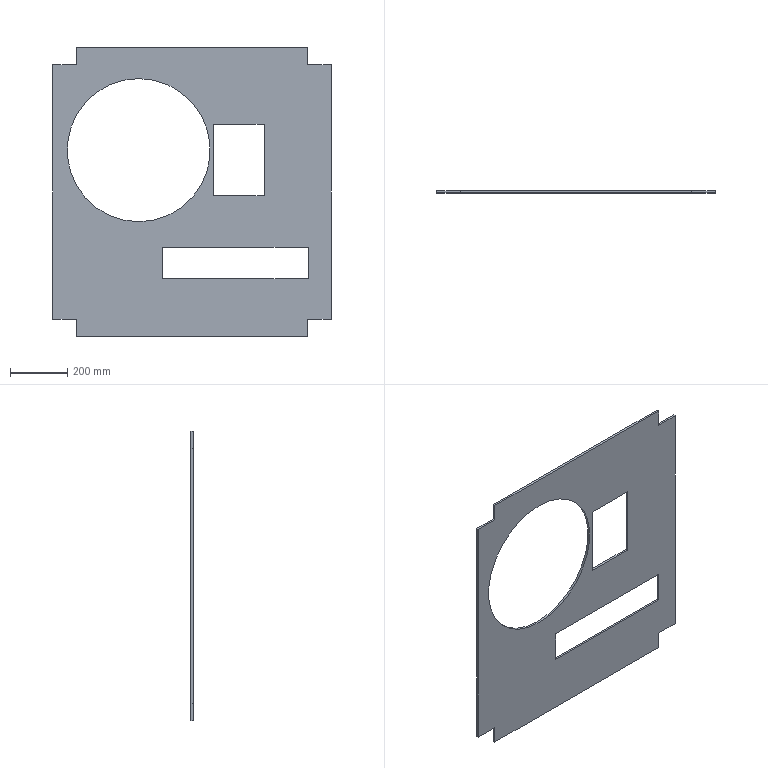Part | STEP file | Guide wheel mechanism revised.sldasm-Part-31 | 1 solid | 24 faces | box 972.42 x 8 x 1012 mm | volume 5346860 mm3 | plane 22 | cylinder 2 | commonest cylinder face diameters 500 x2
STEP:
#1=CARTESIAN_POINT('',(-186.21,820.01,-103.79));
#2=VERTEX_POINT('',#1);
#3=CARTESIAN_POINT('',(-186.21,820.01,396.21));
#4=VERTEX_POINT('',#3);
#5=CARTESIAN_POINT('',(-186.21,820.01,146.21));
#6=DIRECTION('',(0.,1.,0.));
#7=DIRECTION('',(0.,0.,1.));
#8=AXIS2_PLACEMENT_3D('',#5,#6,#7);
#9=CIRCLE('',#8,250.);
#10=EDGE_CURVE('',#2,#4,#9,.T.);
#11=ORIENTED_EDGE('',*,*,#10,.F.);
#12=CARTESIAN_POINT('',(-186.21,828.01,-103.79));
#13=VERTEX_POINT('',#12);
#14=CARTESIAN_POINT('',(-186.21,818.01,-103.79));
#15=DIRECTION('',(0.,1.,0.));
#16=VECTOR('',#15,1000.);
#17=LINE('',#14,#16);
#18=EDGE_CURVE('',#2,#13,#17,.T.);
#19=ORIENTED_EDGE('',*,*,#18,.T.);
#20=CARTESIAN_POINT('',(-186.21,828.01,396.21));
#21=VERTEX_POINT('',#20);
#22=CARTESIAN_POINT('',(-186.21,828.01,146.21));
#23=DIRECTION('',(0.,1.,0.));
#24=DIRECTION('',(0.,0.,1.));
#25=AXIS2_PLACEMENT_3D('',#22,#23,#24);
#26=CIRCLE('',#25,250.);
#27=EDGE_CURVE('',#13,#21,#26,.T.);
#28=ORIENTED_EDGE('',*,*,#27,.T.);
#29=CARTESIAN_POINT('',(-186.21,818.01,396.21));
#30=DIRECTION('',(0.,1.,0.));
#31=VECTOR('',#30,1000.);
#32=LINE('',#29,#31);
#33=EDGE_CURVE('',#4,#21,#32,.T.);
#34=ORIENTED_EDGE('',*,*,#33,.F.);
#35=EDGE_LOOP('',(#11,#19,#28,#34));
#36=FACE_OUTER_BOUND('',#35,.T.);
#37=CARTESIAN_POINT('',(-186.21,818.01,146.21));
#38=DIRECTION('',(0.,1.,0.));
#39=DIRECTION('',(0.,0.,1.));
#40=AXIS2_PLACEMENT_3D('',#37,#38,#39);
#41=CYLINDRICAL_SURFACE('',#40,250.);
#42=ADVANCED_FACE('',(#36),#41,.F.);
#43=CARTESIAN_POINT('',(-404.9,820.01,-506.21));
#44=VERTEX_POINT('',#43);
#45=CARTESIAN_POINT('',(-404.9,820.01,-444.9));
#46=VERTEX_POINT('',#45);
#47=CARTESIAN_POINT('',(-404.9,820.01,-506.21));
#48=DIRECTION('',(0.,0.,1.));
#49=VECTOR('',#48,1000.);
#50=LINE('',#47,#49);
#51=EDGE_CURVE('',#44,#46,#50,.T.);
#52=ORIENTED_EDGE('',*,*,#51,.T.);
#53=CARTESIAN_POINT('',(-404.9,828.01,-444.9));
#54=VERTEX_POINT('',#53);
#55=CARTESIAN_POINT('',(-404.9,828.01,-444.9));
#56=DIRECTION('',(0.,-1.,0.));
#57=VECTOR('',#56,1000.);
#58=LINE('',#55,#57);
#59=EDGE_CURVE('',#54,#46,#58,.T.);
#60=ORIENTED_EDGE('',*,*,#59,.F.);
#61=CARTESIAN_POINT('',(-404.9,828.01,-506.21));
#62=VERTEX_POINT('',#61);
#63=CARTESIAN_POINT('',(-404.9,828.01,-506.21));
#64=DIRECTION('',(0.,0.,1.));
#65=VECTOR('',#64,1000.);
#66=LINE('',#63,#65);
#67=EDGE_CURVE('',#62,#54,#66,.T.);
#68=ORIENTED_EDGE('',*,*,#67,.F.);
#69=CARTESIAN_POINT('',(-404.9,828.01,-506.21));
#70=DIRECTION('',(0.,-1.,0.));
#71=VECTOR('',#70,1000.);
#72=LINE('',#69,#71);
#73=EDGE_CURVE('',#62,#44,#72,.T.);
#74=ORIENTED_EDGE('',*,*,#73,.T.);
#75=EDGE_LOOP('',(#52,#60,#68,#74));
#76=FACE_OUTER_BOUND('',#75,.T.);
#77=CARTESIAN_POINT('',(-404.9,828.01,-506.21));
#78=DIRECTION('',(1.,0.,0.));
#79=DIRECTION('',(0.,0.,-1.));
#80=AXIS2_PLACEMENT_3D('',#77,#78,#79);
#81=PLANE('',#80);
#82=ADVANCED_FACE('',(#76),#81,.F.);
#83=CARTESIAN_POINT('',(-486.21,820.01,-444.9));
#84=VERTEX_POINT('',#83);
#85=CARTESIAN_POINT('',(-404.9,820.01,-444.9));
#86=DIRECTION('',(-1.,0.,0.));
#87=VECTOR('',#86,1000.);
#88=LINE('',#85,#87);
#89=EDGE_CURVE('',#46,#84,#88,.T.);
#90=ORIENTED_EDGE('',*,*,#89,.T.);
#91=CARTESIAN_POINT('',(-486.21,828.01,-444.9));
#92=VERTEX_POINT('',#91);
#93=CARTESIAN_POINT('',(-486.21,828.01,-444.9));
#94=DIRECTION('',(0.,-1.,0.));
#95=VECTOR('',#94,1000.);
#96=LINE('',#93,#95);
#97=EDGE_CURVE('',#92,#84,#96,.T.);
#98=ORIENTED_EDGE('',*,*,#97,.F.);
#99=CARTESIAN_POINT('',(-404.9,828.01,-444.9));
#100=DIRECTION('',(-1.,0.,0.));
#101=VECTOR('',#100,1000.);
#102=LINE('',#99,#101);
#103=EDGE_CURVE('',#54,#92,#102,.T.);
#104=ORIENTED_EDGE('',*,*,#103,.F.);
#105=ORIENTED_EDGE('',*,*,#59,.T.);
#106=EDGE_LOOP('',(#90,#98,#104,#105));
#107=FACE_OUTER_BOUND('',#106,.T.);
#108=CARTESIAN_POINT('',(-404.9,828.01,-444.9));
#109=DIRECTION('',(0.,0.,1.));
#110=DIRECTION('',(1.,0.,0.));
#111=AXIS2_PLACEMENT_3D('',#108,#109,#110);
#112=PLANE('',#111);
#113=ADVANCED_FACE('',(#107),#112,.F.);
#114=CARTESIAN_POINT('',(-486.21,820.01,444.9));
#115=VERTEX_POINT('',#114);
#116=CARTESIAN_POINT('',(-486.21,820.01,-444.9));
#117=DIRECTION('',(0.,0.,1.));
#118=VECTOR('',#117,1000.);
#119=LINE('',#116,#118);
#120=EDGE_CURVE('',#84,#115,#119,.T.);
#121=ORIENTED_EDGE('',*,*,#120,.T.);
#122=CARTESIAN_POINT('',(-486.21,828.01,444.9));
#123=VERTEX_POINT('',#122);
#124=CARTESIAN_POINT('',(-486.21,828.01,444.9));
#125=DIRECTION('',(0.,-1.,0.));
#126=VECTOR('',#125,1000.);
#127=LINE('',#124,#126);
#128=EDGE_CURVE('',#123,#115,#127,.T.);
#129=ORIENTED_EDGE('',*,*,#128,.F.);
#130=CARTESIAN_POINT('',(-486.21,828.01,-444.9));
#131=DIRECTION('',(0.,0.,1.));
#132=VECTOR('',#131,1000.);
#133=LINE('',#130,#132);
#134=EDGE_CURVE('',#92,#123,#133,.T.);
#135=ORIENTED_EDGE('',*,*,#134,.F.);
#136=ORIENTED_EDGE('',*,*,#97,.T.);
#137=EDGE_LOOP('',(#121,#129,#135,#136));
#138=FACE_OUTER_BOUND('',#137,.T.);
#139=CARTESIAN_POINT('',(-486.21,828.01,-444.9));
#140=DIRECTION('',(1.,0.,0.));
#141=DIRECTION('',(0.,0.,-1.));
#142=AXIS2_PLACEMENT_3D('',#139,#140,#141);
#143=PLANE('',#142);
#144=ADVANCED_FACE('',(#138),#143,.F.);
#145=CARTESIAN_POINT('',(-404.9,820.01,444.9));
#146=VERTEX_POINT('',#145);
#147=CARTESIAN_POINT('',(-486.21,820.01,444.9));
#148=DIRECTION('',(1.,0.,0.));
#149=VECTOR('',#148,1000.);
#150=LINE('',#147,#149);
#151=EDGE_CURVE('',#115,#146,#150,.T.);
#152=ORIENTED_EDGE('',*,*,#151,.T.);
#153=CARTESIAN_POINT('',(-404.9,828.01,444.9));
#154=VERTEX_POINT('',#153);
#155=CARTESIAN_POINT('',(-404.9,828.01,444.9));
#156=DIRECTION('',(0.,-1.,0.));
#157=VECTOR('',#156,1000.);
#158=LINE('',#155,#157);
#159=EDGE_CURVE('',#154,#146,#158,.T.);
#160=ORIENTED_EDGE('',*,*,#159,.F.);
#161=CARTESIAN_POINT('',(-486.21,828.01,444.9));
#162=DIRECTION('',(1.,0.,0.));
#163=VECTOR('',#162,1000.);
#164=LINE('',#161,#163);
#165=EDGE_CURVE('',#123,#154,#164,.T.);
#166=ORIENTED_EDGE('',*,*,#165,.F.);
#167=ORIENTED_EDGE('',*,*,#128,.T.);
#168=EDGE_LOOP('',(#152,#160,#166,#167));
#169=FACE_OUTER_BOUND('',#168,.T.);
#170=CARTESIAN_POINT('',(-486.21,828.01,444.9));
#171=DIRECTION('',(0.,0.,-1.));
#172=DIRECTION('',(-1.,0.,0.));
#173=AXIS2_PLACEMENT_3D('',#170,#171,#172);
#174=PLANE('',#173);
#175=ADVANCED_FACE('',(#169),#174,.F.);
#176=CARTESIAN_POINT('',(-404.9,820.01,506.21));
#177=VERTEX_POINT('',#176);
#178=CARTESIAN_POINT('',(-404.9,820.01,444.9));
#179=DIRECTION('',(0.,0.,1.));
#180=VECTOR('',#179,1000.);
#181=LINE('',#178,#180);
#182=EDGE_CURVE('',#146,#177,#181,.T.);
#183=ORIENTED_EDGE('',*,*,#182,.T.);
#184=CARTESIAN_POINT('',(-404.9,828.01,506.21));
#185=VERTEX_POINT('',#184);
#186=CARTESIAN_POINT('',(-404.9,828.01,506.21));
#187=DIRECTION('',(0.,-1.,0.));
#188=VECTOR('',#187,1000.);
#189=LINE('',#186,#188);
#190=EDGE_CURVE('',#185,#177,#189,.T.);
#191=ORIENTED_EDGE('',*,*,#190,.F.);
#192=CARTESIAN_POINT('',(-404.9,828.01,444.9));
#193=DIRECTION('',(0.,0.,1.));
#194=VECTOR('',#193,1000.);
#195=LINE('',#192,#194);
#196=EDGE_CURVE('',#154,#185,#195,.T.);
#197=ORIENTED_EDGE('',*,*,#196,.F.);
#198=ORIENTED_EDGE('',*,*,#159,.T.);
#199=EDGE_LOOP('',(#183,#191,#197,#198));
#200=FACE_OUTER_BOUND('',#199,.T.);
#201=CARTESIAN_POINT('',(-404.9,828.01,444.9));
#202=DIRECTION('',(1.,0.,0.));
#203=DIRECTION('',(0.,0.,-1.));
#204=AXIS2_PLACEMENT_3D('',#201,#202,#203);
#205=PLANE('',#204);
#206=ADVANCED_FACE('',(#200),#205,.F.);
#207=CARTESIAN_POINT('',(404.9,820.01,506.21));
#208=VERTEX_POINT('',#207);
#209=CARTESIAN_POINT('',(0.,820.01,506.21));
#210=DIRECTION('',(1.,0.,0.));
#211=VECTOR('',#210,1000.);
#212=LINE('',#209,#211);
#213=EDGE_CURVE('',#177,#208,#212,.T.);
#214=ORIENTED_EDGE('',*,*,#213,.T.);
#215=CARTESIAN_POINT('',(404.9,828.01,506.21));
#216=VERTEX_POINT('',#215);
#217=CARTESIAN_POINT('',(404.9,828.01,506.21));
#218=DIRECTION('',(0.,-1.,0.));
#219=VECTOR('',#218,1000.);
#220=LINE('',#217,#219);
#221=EDGE_CURVE('',#216,#208,#220,.T.);
#222=ORIENTED_EDGE('',*,*,#221,.F.);
#223=CARTESIAN_POINT('',(-404.9,828.01,506.21));
#224=DIRECTION('',(1.,0.,0.));
#225=VECTOR('',#224,1000.);
#226=LINE('',#223,#225);
#227=EDGE_CURVE('',#185,#216,#226,.T.);
#228=ORIENTED_EDGE('',*,*,#227,.F.);
#229=ORIENTED_EDGE('',*,*,#190,.T.);
#230=EDGE_LOOP('',(#214,#222,#228,#229));
#231=FACE_OUTER_BOUND('',#230,.T.);
#232=CARTESIAN_POINT('',(0.,828.01,506.21));
#233=DIRECTION('',(0.,0.,-1.));
#234=DIRECTION('',(-1.,0.,0.));
#235=AXIS2_PLACEMENT_3D('',#232,#233,#234);
#236=PLANE('',#235);
#237=ADVANCED_FACE('',(#231),#236,.F.);
#238=CARTESIAN_POINT('',(404.9,820.01,444.9));
#239=VERTEX_POINT('',#238);
#240=CARTESIAN_POINT('',(404.9,820.01,506.21));
#241=DIRECTION('',(0.,0.,-1.));
#242=VECTOR('',#241,1000.);
#243=LINE('',#240,#242);
#244=EDGE_CURVE('',#208,#239,#243,.T.);
#245=ORIENTED_EDGE('',*,*,#244,.T.);
#246=CARTESIAN_POINT('',(404.9,828.01,444.9));
#247=VERTEX_POINT('',#246);
#248=CARTESIAN_POINT('',(404.9,828.01,444.9));
#249=DIRECTION('',(0.,-1.,0.));
#250=VECTOR('',#249,1000.);
#251=LINE('',#248,#250);
#252=EDGE_CURVE('',#247,#239,#251,.T.);
#253=ORIENTED_EDGE('',*,*,#252,.F.);
#254=CARTESIAN_POINT('',(404.9,828.01,506.21));
#255=DIRECTION('',(0.,0.,-1.));
#256=VECTOR('',#255,1000.);
#257=LINE('',#254,#256);
#258=EDGE_CURVE('',#216,#247,#257,.T.);
#259=ORIENTED_EDGE('',*,*,#258,.F.);
#260=ORIENTED_EDGE('',*,*,#221,.T.);
#261=EDGE_LOOP('',(#245,#253,#259,#260));
#262=FACE_OUTER_BOUND('',#261,.T.);
#263=CARTESIAN_POINT('',(404.9,828.01,506.21));
#264=DIRECTION('',(-1.,0.,0.));
#265=DIRECTION('',(0.,0.,1.));
#266=AXIS2_PLACEMENT_3D('',#263,#264,#265);
#267=PLANE('',#266);
#268=ADVANCED_FACE('',(#262),#267,.F.);
#269=CARTESIAN_POINT('',(486.21,820.01,444.9));
#270=VERTEX_POINT('',#269);
#271=CARTESIAN_POINT('',(404.9,820.01,444.9));
#272=DIRECTION('',(1.,0.,0.));
#273=VECTOR('',#272,1000.);
#274=LINE('',#271,#273);
#275=EDGE_CURVE('',#239,#270,#274,.T.);
#276=ORIENTED_EDGE('',*,*,#275,.T.);
#277=CARTESIAN_POINT('',(486.21,828.01,444.9));
#278=VERTEX_POINT('',#277);
#279=CARTESIAN_POINT('',(486.21,828.01,444.9));
#280=DIRECTION('',(0.,-1.,0.));
#281=VECTOR('',#280,1000.);
#282=LINE('',#279,#281);
#283=EDGE_CURVE('',#278,#270,#282,.T.);
#284=ORIENTED_EDGE('',*,*,#283,.F.);
#285=CARTESIAN_POINT('',(404.9,828.01,444.9));
#286=DIRECTION('',(1.,0.,0.));
#287=VECTOR('',#286,1000.);
#288=LINE('',#285,#287);
#289=EDGE_CURVE('',#247,#278,#288,.T.);
#290=ORIENTED_EDGE('',*,*,#289,.F.);
#291=ORIENTED_EDGE('',*,*,#252,.T.);
#292=EDGE_LOOP('',(#276,#284,#290,#291));
#293=FACE_OUTER_BOUND('',#292,.T.);
#294=CARTESIAN_POINT('',(404.9,828.01,444.9));
#295=DIRECTION('',(0.,0.,-1.));
#296=DIRECTION('',(-1.,0.,0.));
#297=AXIS2_PLACEMENT_3D('',#294,#295,#296);
#298=PLANE('',#297);
#299=ADVANCED_FACE('',(#293),#298,.F.);
#300=CARTESIAN_POINT('',(486.21,820.01,-444.9));
#301=VERTEX_POINT('',#300);
#302=CARTESIAN_POINT('',(486.21,820.01,444.9));
#303=DIRECTION('',(0.,0.,-1.));
#304=VECTOR('',#303,1000.);
#305=LINE('',#302,#304);
#306=EDGE_CURVE('',#270,#301,#305,.T.);
#307=ORIENTED_EDGE('',*,*,#306,.T.);
#308=CARTESIAN_POINT('',(486.21,828.01,-444.9));
#309=VERTEX_POINT('',#308);
#310=CARTESIAN_POINT('',(486.21,828.01,-444.9));
#311=DIRECTION('',(0.,-1.,0.));
#312=VECTOR('',#311,1000.);
#313=LINE('',#310,#312);
#314=EDGE_CURVE('',#309,#301,#313,.T.);
#315=ORIENTED_EDGE('',*,*,#314,.F.);
#316=CARTESIAN_POINT('',(486.21,828.01,444.9));
#317=DIRECTION('',(0.,0.,-1.));
#318=VECTOR('',#317,1000.);
#319=LINE('',#316,#318);
#320=EDGE_CURVE('',#278,#309,#319,.T.);
#321=ORIENTED_EDGE('',*,*,#320,.F.);
#322=ORIENTED_EDGE('',*,*,#283,.T.);
#323=EDGE_LOOP('',(#307,#315,#321,#322));
#324=FACE_OUTER_BOUND('',#323,.T.);
#325=CARTESIAN_POINT('',(486.21,828.01,444.9));
#326=DIRECTION('',(-1.,0.,0.));
#327=DIRECTION('',(0.,0.,1.));
#328=AXIS2_PLACEMENT_3D('',#325,#326,#327);
#329=PLANE('',#328);
#330=ADVANCED_FACE('',(#324),#329,.F.);
#331=CARTESIAN_POINT('',(404.9,820.01,-444.9));
#332=VERTEX_POINT('',#331);
#333=CARTESIAN_POINT('',(486.21,820.01,-444.9));
#334=DIRECTION('',(-1.,0.,0.));
#335=VECTOR('',#334,1000.);
#336=LINE('',#333,#335);
#337=EDGE_CURVE('',#301,#332,#336,.T.);
#338=ORIENTED_EDGE('',*,*,#337,.T.);
#339=CARTESIAN_POINT('',(404.9,828.01,-444.9));
#340=VERTEX_POINT('',#339);
#341=CARTESIAN_POINT('',(404.9,828.01,-444.9));
#342=DIRECTION('',(0.,-1.,0.));
#343=VECTOR('',#342,1000.);
#344=LINE('',#341,#343);
#345=EDGE_CURVE('',#340,#332,#344,.T.);
#346=ORIENTED_EDGE('',*,*,#345,.F.);
#347=CARTESIAN_POINT('',(486.21,828.01,-444.9));
#348=DIRECTION('',(-1.,0.,0.));
#349=VECTOR('',#348,1000.);
#350=LINE('',#347,#349);
#351=EDGE_CURVE('',#309,#340,#350,.T.);
#352=ORIENTED_EDGE('',*,*,#351,.F.);
#353=ORIENTED_EDGE('',*,*,#314,.T.);
#354=EDGE_LOOP('',(#338,#346,#352,#353));
#355=FACE_OUTER_BOUND('',#354,.T.);
#356=CARTESIAN_POINT('',(486.21,828.01,-444.9));
#357=DIRECTION('',(0.,0.,1.));
#358=DIRECTION('',(1.,0.,0.));
#359=AXIS2_PLACEMENT_3D('',#356,#357,#358);
#360=PLANE('',#359);
#361=ADVANCED_FACE('',(#355),#360,.F.);
#362=CARTESIAN_POINT('',(404.9,820.01,-506.21));
#363=VERTEX_POINT('',#362);
#364=CARTESIAN_POINT('',(404.9,820.01,-444.9));
#365=DIRECTION('',(0.,0.,-1.));
#366=VECTOR('',#365,1000.);
#367=LINE('',#364,#366);
#368=EDGE_CURVE('',#332,#363,#367,.T.);
#369=ORIENTED_EDGE('',*,*,#368,.T.);
#370=CARTESIAN_POINT('',(404.9,828.01,-506.21));
#371=VERTEX_POINT('',#370);
#372=CARTESIAN_POINT('',(404.9,828.01,-506.21));
#373=DIRECTION('',(0.,-1.,0.));
#374=VECTOR('',#373,1000.);
#375=LINE('',#372,#374);
#376=EDGE_CURVE('',#371,#363,#375,.T.);
#377=ORIENTED_EDGE('',*,*,#376,.F.);
#378=CARTESIAN_POINT('',(404.9,828.01,-444.9));
#379=DIRECTION('',(0.,0.,-1.));
#380=VECTOR('',#379,1000.);
#381=LINE('',#378,#380);
#382=EDGE_CURVE('',#340,#371,#381,.T.);
#383=ORIENTED_EDGE('',*,*,#382,.F.);
#384=ORIENTED_EDGE('',*,*,#345,.T.);
#385=EDGE_LOOP('',(#369,#377,#383,#384));
#386=FACE_OUTER_BOUND('',#385,.T.);
#387=CARTESIAN_POINT('',(404.9,828.01,-444.9));
#388=DIRECTION('',(-1.,0.,0.));
#389=DIRECTION('',(0.,0.,1.));
#390=AXIS2_PLACEMENT_3D('',#387,#388,#389);
#391=PLANE('',#390);
#392=ADVANCED_FACE('',(#386),#391,.F.);
#393=CARTESIAN_POINT('',(0.,820.01,-506.21));
#394=DIRECTION('',(-1.,0.,0.));
#395=VECTOR('',#394,1000.);
#396=LINE('',#393,#395);
#397=EDGE_CURVE('',#363,#44,#396,.T.);
#398=ORIENTED_EDGE('',*,*,#397,.T.);
#399=ORIENTED_EDGE('',*,*,#73,.F.);
#400=CARTESIAN_POINT('',(0.,828.01,-506.21));
#401=DIRECTION('',(-1.,0.,0.));
#402=VECTOR('',#401,1000.);
#403=LINE('',#400,#402);
#404=EDGE_CURVE('',#371,#62,#403,.T.);
#405=ORIENTED_EDGE('',*,*,#404,.F.);
#406=ORIENTED_EDGE('',*,*,#376,.T.);
#407=EDGE_LOOP('',(#398,#399,#405,#406));
#408=FACE_OUTER_BOUND('',#407,.T.);
#409=CARTESIAN_POINT('',(0.,828.01,-506.21));
#410=DIRECTION('',(0.,0.,1.));
#411=DIRECTION('',(1.,0.,0.));
#412=AXIS2_PLACEMENT_3D('',#409,#410,#411);
#413=PLANE('',#412);
#414=ADVANCED_FACE('',(#408),#413,.F.);
#415=CARTESIAN_POINT('',(76.71,828.01,-12.79));
#416=VERTEX_POINT('',#415);
#417=CARTESIAN_POINT('',(76.71,828.01,237.21));
#418=VERTEX_POINT('',#417);
#419=CARTESIAN_POINT('',(76.71,828.01,-12.79));
#420=DIRECTION('',(0.,0.,1.));
#421=VECTOR('',#420,1000.);
#422=LINE('',#419,#421);
#423=EDGE_CURVE('',#416,#418,#422,.T.);
#424=ORIENTED_EDGE('',*,*,#423,.F.);
#425=CARTESIAN_POINT('',(251.71,828.01,-12.79));
#426=VERTEX_POINT('',#425);
#427=CARTESIAN_POINT('',(76.71,828.01,-12.79));
#428=DIRECTION('',(-1.,0.,0.));
#429=VECTOR('',#428,1000.);
#430=LINE('',#427,#429);
#431=EDGE_CURVE('',#426,#416,#430,.T.);
#432=ORIENTED_EDGE('',*,*,#431,.F.);
#433=CARTESIAN_POINT('',(251.71,828.01,237.21));
#434=VERTEX_POINT('',#433);
#435=CARTESIAN_POINT('',(251.71,828.01,-12.79));
#436=DIRECTION('',(0.,0.,-1.));
#437=VECTOR('',#436,1000.);
#438=LINE('',#435,#437);
#439=EDGE_CURVE('',#434,#426,#438,.T.);
#440=ORIENTED_EDGE('',*,*,#439,.F.);
#441=CARTESIAN_POINT('',(76.71,828.01,237.21));
#442=DIRECTION('',(1.,0.,0.));
#443=VECTOR('',#442,1000.);
#444=LINE('',#441,#443);
#445=EDGE_CURVE('',#418,#434,#444,.T.);
#446=ORIENTED_EDGE('',*,*,#445,.F.);
#447=EDGE_LOOP('',(#424,#432,#440,#446));
#448=FACE_BOUND('',#447,.T.);
#449=CARTESIAN_POINT('',(406.21,828.01,-193.79));
#450=VERTEX_POINT('',#449);
#451=CARTESIAN_POINT('',(406.21,828.01,-303.79));
#452=VERTEX_POINT('',#451);
#453=CARTESIAN_POINT('',(406.21,828.01,-303.79));
#454=DIRECTION('',(0.,0.,-1.));
#455=VECTOR('',#454,1000.);
#456=LINE('',#453,#455);
#457=EDGE_CURVE('',#450,#452,#456,.T.);
#458=ORIENTED_EDGE('',*,*,#457,.F.);
#459=CARTESIAN_POINT('',(-103.79,828.01,-193.79));
#460=VERTEX_POINT('',#459);
#461=CARTESIAN_POINT('',(406.21,828.01,-193.79));
#462=DIRECTION('',(1.,0.,0.));
#463=VECTOR('',#462,1000.);
#464=LINE('',#461,#463);
#465=EDGE_CURVE('',#460,#450,#464,.T.);
#466=ORIENTED_EDGE('',*,*,#465,.F.);
#467=CARTESIAN_POINT('',(-103.79,828.01,-303.79));
#468=VERTEX_POINT('',#467);
#469=CARTESIAN_POINT('',(-103.79,828.01,-303.79));
#470=DIRECTION('',(0.,0.,1.));
#471=VECTOR('',#470,1000.);
#472=LINE('',#469,#471);
#473=EDGE_CURVE('',#468,#460,#472,.T.);
#474=ORIENTED_EDGE('',*,*,#473,.F.);
#475=CARTESIAN_POINT('',(406.21,828.01,-303.79));
#476=DIRECTION('',(-1.,0.,0.));
#477=VECTOR('',#476,1000.);
#478=LINE('',#475,#477);
#479=EDGE_CURVE('',#452,#468,#478,.T.);
#480=ORIENTED_EDGE('',*,*,#479,.F.);
#481=EDGE_LOOP('',(#458,#466,#474,#480));
#482=FACE_BOUND('',#481,.T.);
#483=CARTESIAN_POINT('',(-186.21,828.01,146.21));
#484=DIRECTION('',(0.,1.,0.));
#485=DIRECTION('',(0.,0.,1.));
#486=AXIS2_PLACEMENT_3D('',#483,#484,#485);
#487=CIRCLE('',#486,250.);
#488=EDGE_CURVE('',#21,#13,#487,.T.);
#489=ORIENTED_EDGE('',*,*,#488,.F.);
#490=ORIENTED_EDGE('',*,*,#27,.F.);
#491=EDGE_LOOP('',(#489,#490));
#492=FACE_BOUND('',#491,.T.);
#493=ORIENTED_EDGE('',*,*,#404,.T.);
#494=ORIENTED_EDGE('',*,*,#67,.T.);
#495=ORIENTED_EDGE('',*,*,#103,.T.);
#496=ORIENTED_EDGE('',*,*,#134,.T.);
#497=ORIENTED_EDGE('',*,*,#165,.T.);
#498=ORIENTED_EDGE('',*,*,#196,.T.);
#499=ORIENTED_EDGE('',*,*,#227,.T.);
#500=ORIENTED_EDGE('',*,*,#258,.T.);
#501=ORIENTED_EDGE('',*,*,#289,.T.);
#502=ORIENTED_EDGE('',*,*,#320,.T.);
#503=ORIENTED_EDGE('',*,*,#351,.T.);
#504=ORIENTED_EDGE('',*,*,#382,.T.);
#505=EDGE_LOOP('',(#493,#494,#495,#496,#497,#498,#499,#500,#501,#502,#503,#504));
#506=FACE_OUTER_BOUND('',#505,.T.);
#507=CARTESIAN_POINT('',(0.,828.01,0.));
#508=DIRECTION('',(0.,1.,0.));
#509=DIRECTION('',(0.,0.,1.));
#510=AXIS2_PLACEMENT_3D('',#507,#508,#509);
#511=PLANE('',#510);
#512=ADVANCED_FACE('',(#448,#482,#492,#506),#511,.T.);
#513=CARTESIAN_POINT('',(76.71,820.01,-12.79));
#514=VERTEX_POINT('',#513);
#515=CARTESIAN_POINT('',(251.71,820.01,-12.79));
#516=VERTEX_POINT('',#515);
#517=CARTESIAN_POINT('',(76.71,820.01,-12.79));
#518=DIRECTION('',(1.,0.,0.));
#519=VECTOR('',#518,1000.);
#520=LINE('',#517,#519);
#521=EDGE_CURVE('',#514,#516,#520,.T.);
#522=ORIENTED_EDGE('',*,*,#521,.F.);
#523=CARTESIAN_POINT('',(76.71,820.01,237.21));
#524=VERTEX_POINT('',#523);
#525=CARTESIAN_POINT('',(76.71,820.01,-12.79));
#526=DIRECTION('',(0.,0.,-1.));
#527=VECTOR('',#526,1000.);
#528=LINE('',#525,#527);
#529=EDGE_CURVE('',#524,#514,#528,.T.);
#530=ORIENTED_EDGE('',*,*,#529,.F.);
#531=CARTESIAN_POINT('',(251.71,820.01,237.21));
#532=VERTEX_POINT('',#531);
#533=CARTESIAN_POINT('',(76.71,820.01,237.21));
#534=DIRECTION('',(-1.,0.,0.));
#535=VECTOR('',#534,1000.);
#536=LINE('',#533,#535);
#537=EDGE_CURVE('',#532,#524,#536,.T.);
#538=ORIENTED_EDGE('',*,*,#537,.F.);
#539=CARTESIAN_POINT('',(251.71,820.01,-12.79));
#540=DIRECTION('',(0.,0.,1.));
#541=VECTOR('',#540,1000.);
#542=LINE('',#539,#541);
#543=EDGE_CURVE('',#516,#532,#542,.T.);
#544=ORIENTED_EDGE('',*,*,#543,.F.);
#545=EDGE_LOOP('',(#522,#530,#538,#544));
#546=FACE_BOUND('',#545,.T.);
#547=CARTESIAN_POINT('',(406.21,820.01,-193.79));
#548=VERTEX_POINT('',#547);
#549=CARTESIAN_POINT('',(-103.79,820.01,-193.79));
#550=VERTEX_POINT('',#549);
#551=CARTESIAN_POINT('',(406.21,820.01,-193.79));
#552=DIRECTION('',(-1.,0.,0.));
#553=VECTOR('',#552,1000.);
#554=LINE('',#551,#553);
#555=EDGE_CURVE('',#548,#550,#554,.T.);
#556=ORIENTED_EDGE('',*,*,#555,.F.);
#557=CARTESIAN_POINT('',(406.21,820.01,-303.79));
#558=VERTEX_POINT('',#557);
#559=CARTESIAN_POINT('',(406.21,820.01,-303.79));
#560=DIRECTION('',(0.,0.,1.));
#561=VECTOR('',#560,1000.);
#562=LINE('',#559,#561);
#563=EDGE_CURVE('',#558,#548,#562,.T.);
#564=ORIENTED_EDGE('',*,*,#563,.F.);
#565=CARTESIAN_POINT('',(-103.79,820.01,-303.79));
#566=VERTEX_POINT('',#565);
#567=CARTESIAN_POINT('',(406.21,820.01,-303.79));
#568=DIRECTION('',(1.,0.,0.));
#569=VECTOR('',#568,1000.);
#570=LINE('',#567,#569);
#571=EDGE_CURVE('',#566,#558,#570,.T.);
#572=ORIENTED_EDGE('',*,*,#571,.F.);
#573=CARTESIAN_POINT('',(-103.79,820.01,-303.79));
#574=DIRECTION('',(0.,0.,-1.));
#575=VECTOR('',#574,1000.);
#576=LINE('',#573,#575);
#577=EDGE_CURVE('',#550,#566,#576,.T.);
#578=ORIENTED_EDGE('',*,*,#577,.F.);
#579=EDGE_LOOP('',(#556,#564,#572,#578));
#580=FACE_BOUND('',#579,.T.);
#581=CARTESIAN_POINT('',(-186.21,820.01,146.21));
#582=DIRECTION('',(0.,1.,0.));
#583=DIRECTION('',(0.,0.,1.));
#584=AXIS2_PLACEMENT_3D('',#581,#582,#583);
#585=CIRCLE('',#584,250.);
#586=EDGE_CURVE('',#4,#2,#585,.T.);
#587=ORIENTED_EDGE('',*,*,#586,.T.);
#588=ORIENTED_EDGE('',*,*,#10,.T.);
#589=EDGE_LOOP('',(#587,#588));
#590=FACE_BOUND('',#589,.T.);
#591=ORIENTED_EDGE('',*,*,#51,.F.);
#592=ORIENTED_EDGE('',*,*,#397,.F.);
#593=ORIENTED_EDGE('',*,*,#368,.F.);
#594=ORIENTED_EDGE('',*,*,#337,.F.);
#595=ORIENTED_EDGE('',*,*,#306,.F.);
#596=ORIENTED_EDGE('',*,*,#275,.F.);
#597=ORIENTED_EDGE('',*,*,#244,.F.);
#598=ORIENTED_EDGE('',*,*,#213,.F.);
#599=ORIENTED_EDGE('',*,*,#182,.F.);
#600=ORIENTED_EDGE('',*,*,#151,.F.);
#601=ORIENTED_EDGE('',*,*,#120,.F.);
#602=ORIENTED_EDGE('',*,*,#89,.F.);
#603=EDGE_LOOP('',(#591,#592,#593,#594,#595,#596,#597,#598,#599,#600,#601,#602));
#604=FACE_OUTER_BOUND('',#603,.T.);
#605=CARTESIAN_POINT('',(0.,820.01,0.));
#606=DIRECTION('',(0.,1.,0.));
#607=DIRECTION('',(0.,0.,1.));
#608=AXIS2_PLACEMENT_3D('',#605,#606,#607);
#609=PLANE('',#608);
#610=ADVANCED_FACE('',(#546,#580,#590,#604),#609,.F.);
#611=ORIENTED_EDGE('',*,*,#18,.F.);
#612=ORIENTED_EDGE('',*,*,#586,.F.);
#613=ORIENTED_EDGE('',*,*,#33,.T.);
#614=ORIENTED_EDGE('',*,*,#488,.T.);
#615=EDGE_LOOP('',(#611,#612,#613,#614));
#616=FACE_OUTER_BOUND('',#615,.T.);
#617=CARTESIAN_POINT('',(-186.21,818.01,146.21));
#618=DIRECTION('',(0.,1.,0.));
#619=DIRECTION('',(0.,0.,1.));
#620=AXIS2_PLACEMENT_3D('',#617,#618,#619);
#621=CYLINDRICAL_SURFACE('',#620,250.);
#622=ADVANCED_FACE('',(#616),#621,.F.);
#623=ORIENTED_EDGE('',*,*,#563,.T.);
#624=CARTESIAN_POINT('',(406.21,-60.001,-193.79));
#625=DIRECTION('',(0.,1.,0.));
#626=VECTOR('',#625,1000.);
#627=LINE('',#624,#626);
#628=EDGE_CURVE('',#548,#450,#627,.T.);
#629=ORIENTED_EDGE('',*,*,#628,.T.);
#630=ORIENTED_EDGE('',*,*,#457,.T.);
#631=CARTESIAN_POINT('',(406.21,-60.001,-303.79));
#632=DIRECTION('',(0.,1.,0.));
#633=VECTOR('',#632,1000.);
#634=LINE('',#631,#633);
#635=EDGE_CURVE('',#558,#452,#634,.T.);
#636=ORIENTED_EDGE('',*,*,#635,.F.);
#637=EDGE_LOOP('',(#623,#629,#630,#636));
#638=FACE_OUTER_BOUND('',#637,.T.);
#639=CARTESIAN_POINT('',(406.21,-60.001,-303.79));
#640=DIRECTION('',(1.,0.,0.));
#641=DIRECTION('',(0.,0.,-1.));
#642=AXIS2_PLACEMENT_3D('',#639,#640,#641);
#643=PLANE('',#642);
#644=ADVANCED_FACE('',(#638),#643,.F.);
#645=ORIENTED_EDGE('',*,*,#555,.T.);
#646=CARTESIAN_POINT('',(-103.79,-60.001,-193.79));
#647=DIRECTION('',(0.,1.,0.));
#648=VECTOR('',#647,1000.);
#649=LINE('',#646,#648);
#650=EDGE_CURVE('',#550,#460,#649,.T.);
#651=ORIENTED_EDGE('',*,*,#650,.T.);
#652=ORIENTED_EDGE('',*,*,#465,.T.);
#653=ORIENTED_EDGE('',*,*,#628,.F.);
#654=EDGE_LOOP('',(#645,#651,#652,#653));
#655=FACE_OUTER_BOUND('',#654,.T.);
#656=CARTESIAN_POINT('',(406.21,-60.001,-193.79));
#657=DIRECTION('',(0.,0.,1.));
#658=DIRECTION('',(1.,0.,0.));
#659=AXIS2_PLACEMENT_3D('',#656,#657,#658);
#660=PLANE('',#659);
#661=ADVANCED_FACE('',(#655),#660,.F.);
#662=ORIENTED_EDGE('',*,*,#577,.T.);
#663=CARTESIAN_POINT('',(-103.79,-60.001,-303.79));
#664=DIRECTION('',(0.,1.,0.));
#665=VECTOR('',#664,1000.);
#666=LINE('',#663,#665);
#667=EDGE_CURVE('',#566,#468,#666,.T.);
#668=ORIENTED_EDGE('',*,*,#667,.T.);
#669=ORIENTED_EDGE('',*,*,#473,.T.);
#670=ORIENTED_EDGE('',*,*,#650,.F.);
#671=EDGE_LOOP('',(#662,#668,#669,#670));
#672=FACE_OUTER_BOUND('',#671,.T.);
#673=CARTESIAN_POINT('',(-103.79,-60.001,-303.79));
#674=DIRECTION('',(-1.,0.,0.));
#675=DIRECTION('',(0.,0.,1.));
#676=AXIS2_PLACEMENT_3D('',#673,#674,#675);
#677=PLANE('',#676);
#678=ADVANCED_FACE('',(#672),#677,.F.);
#679=ORIENTED_EDGE('',*,*,#571,.T.);
#680=ORIENTED_EDGE('',*,*,#635,.T.);
#681=ORIENTED_EDGE('',*,*,#479,.T.);
#682=ORIENTED_EDGE('',*,*,#667,.F.);
#683=EDGE_LOOP('',(#679,#680,#681,#682));
#684=FACE_OUTER_BOUND('',#683,.T.);
#685=CARTESIAN_POINT('',(406.21,-60.001,-303.79));
#686=DIRECTION('',(0.,0.,-1.));
#687=DIRECTION('',(-1.,0.,0.));
#688=AXIS2_PLACEMENT_3D('',#685,#686,#687);
#689=PLANE('',#688);
#690=ADVANCED_FACE('',(#684),#689,.F.);
#691=ORIENTED_EDGE('',*,*,#529,.T.);
#692=CARTESIAN_POINT('',(76.71,-60.001,-12.79));
#693=DIRECTION('',(0.,1.,0.));
#694=VECTOR('',#693,1000.);
#695=LINE('',#692,#694);
#696=EDGE_CURVE('',#514,#416,#695,.T.);
#697=ORIENTED_EDGE('',*,*,#696,.T.);
#698=ORIENTED_EDGE('',*,*,#423,.T.);
#699=CARTESIAN_POINT('',(76.71,-60.001,237.21));
#700=DIRECTION('',(0.,1.,0.));
#701=VECTOR('',#700,1000.);
#702=LINE('',#699,#701);
#703=EDGE_CURVE('',#524,#418,#702,.T.);
#704=ORIENTED_EDGE('',*,*,#703,.F.);
#705=EDGE_LOOP('',(#691,#697,#698,#704));
#706=FACE_OUTER_BOUND('',#705,.T.);
#707=CARTESIAN_POINT('',(76.71,-60.001,-12.79));
#708=DIRECTION('',(-1.,0.,0.));
#709=DIRECTION('',(0.,0.,1.));
#710=AXIS2_PLACEMENT_3D('',#707,#708,#709);
#711=PLANE('',#710);
#712=ADVANCED_FACE('',(#706),#711,.F.);
#713=ORIENTED_EDGE('',*,*,#521,.T.);
#714=CARTESIAN_POINT('',(251.71,-60.001,-12.79));
#715=DIRECTION('',(0.,1.,0.));
#716=VECTOR('',#715,1000.);
#717=LINE('',#714,#716);
#718=EDGE_CURVE('',#516,#426,#717,.T.);
#719=ORIENTED_EDGE('',*,*,#718,.T.);
#720=ORIENTED_EDGE('',*,*,#431,.T.);
#721=ORIENTED_EDGE('',*,*,#696,.F.);
#722=EDGE_LOOP('',(#713,#719,#720,#721));
#723=FACE_OUTER_BOUND('',#722,.T.);
#724=CARTESIAN_POINT('',(76.71,-60.001,-12.79));
#725=DIRECTION('',(0.,0.,-1.));
#726=DIRECTION('',(-1.,0.,0.));
#727=AXIS2_PLACEMENT_3D('',#724,#725,#726);
#728=PLANE('',#727);
#729=ADVANCED_FACE('',(#723),#728,.F.);
#730=ORIENTED_EDGE('',*,*,#543,.T.);
#731=CARTESIAN_POINT('',(251.71,-60.001,237.21));
#732=DIRECTION('',(0.,1.,0.));
#733=VECTOR('',#732,1000.);
#734=LINE('',#731,#733);
#735=EDGE_CURVE('',#532,#434,#734,.T.);
#736=ORIENTED_EDGE('',*,*,#735,.T.);
#737=ORIENTED_EDGE('',*,*,#439,.T.);
#738=ORIENTED_EDGE('',*,*,#718,.F.);
#739=EDGE_LOOP('',(#730,#736,#737,#738));
#740=FACE_OUTER_BOUND('',#739,.T.);
#741=CARTESIAN_POINT('',(251.71,-60.001,-12.79));
#742=DIRECTION('',(1.,0.,0.));
#743=DIRECTION('',(0.,0.,-1.));
#744=AXIS2_PLACEMENT_3D('',#741,#742,#743);
#745=PLANE('',#744);
#746=ADVANCED_FACE('',(#740),#745,.F.);
#747=ORIENTED_EDGE('',*,*,#537,.T.);
#748=ORIENTED_EDGE('',*,*,#703,.T.);
#749=ORIENTED_EDGE('',*,*,#445,.T.);
#750=ORIENTED_EDGE('',*,*,#735,.F.);
#751=EDGE_LOOP('',(#747,#748,#749,#750));
#752=FACE_OUTER_BOUND('',#751,.T.);
#753=CARTESIAN_POINT('',(76.71,-60.001,237.21));
#754=DIRECTION('',(0.,0.,1.));
#755=DIRECTION('',(1.,0.,0.));
#756=AXIS2_PLACEMENT_3D('',#753,#754,#755);
#757=PLANE('',#756);
#758=ADVANCED_FACE('',(#752),#757,.F.);
#759=CLOSED_SHELL('',(#42,#82,#113,#144,#175,#206,#237,#268,#299,#330,#361,#392,#414,#512,#610,#622,#644,#661,#678,#690,#712,#729,#746,#758));
#760=MANIFOLD_SOLID_BREP('',#759);
#761=CARTESIAN_POINT('',(0.,0.,0.));
#762=DIRECTION('',(0.,0.,1.));
#763=DIRECTION('',(1.,0.,0.));
#764=AXIS2_PLACEMENT_3D('',#761,#762,#763);
#765=(LENGTH_UNIT()NAMED_UNIT(*)SI_UNIT(.MILLI.,.METRE.));
#766=UNCERTAINTY_MEASURE_WITH_UNIT(LENGTH_MEASURE(0.00001),#765,'','');
#767=(NAMED_UNIT(*)PLANE_ANGLE_UNIT()SI_UNIT($,.RADIAN.));
#768=(NAMED_UNIT(*)SI_UNIT($,.STERADIAN.)SOLID_ANGLE_UNIT());
#769=(GEOMETRIC_REPRESENTATION_CONTEXT(3)GLOBAL_UNCERTAINTY_ASSIGNED_CONTEXT((#766))GLOBAL_UNIT_ASSIGNED_CONTEXT((#765,#767,#768))REPRESENTATION_CONTEXT('',''));
#770=ADVANCED_BREP_SHAPE_REPRESENTATION('',(#760,#764),#769);